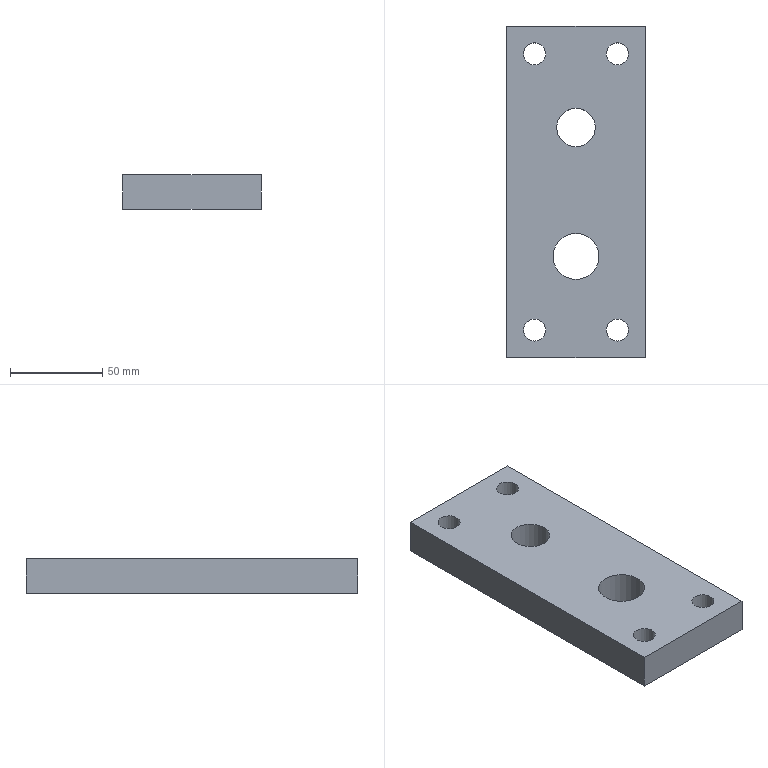Part | NX | features solid 2 | 1 solid | 12 faces | box 75 x 180 x 19 mm | volume 231997 mm3 | plane 6 | cylinder 6 | commonest cylinder face diameters 12 x4 21 x1 25 x1
STEP:
#1=CARTESIAN_POINT('',(-630.,-106.,-55.));
#2=VERTEX_POINT('',#1);
#3=CARTESIAN_POINT('',(-630.,-100.,-55.));
#4=DIRECTION('',(0.,0.,1.));
#5=DIRECTION('',(0.,-1.,0.));
#6=AXIS2_PLACEMENT_3D('',#3,#4,#5);
#7=CIRCLE('',#6,6.);
#8=EDGE_CURVE('',#2,#2,#7,.T.);
#9=ORIENTED_EDGE('',*,*,#8,.F.);
#10=EDGE_LOOP('',(#9));
#11=FACE_BOUND('',#10,.T.);
#12=CARTESIAN_POINT('',(-652.5,-197.5,-55.));
#13=VERTEX_POINT('',#12);
#14=CARTESIAN_POINT('',(-652.5,-210.,-55.));
#15=DIRECTION('',(0.,0.,1.));
#16=DIRECTION('',(0.,1.,0.));
#17=AXIS2_PLACEMENT_3D('',#14,#15,#16);
#18=CIRCLE('',#17,12.5);
#19=EDGE_CURVE('',#13,#13,#18,.T.);
#20=ORIENTED_EDGE('',*,*,#19,.F.);
#21=EDGE_LOOP('',(#20));
#22=FACE_BOUND('',#21,.T.);
#23=CARTESIAN_POINT('',(-652.5,-129.5,-55.));
#24=VERTEX_POINT('',#23);
#25=CARTESIAN_POINT('',(-652.5,-140.,-55.));
#26=DIRECTION('',(0.,0.,1.));
#27=DIRECTION('',(0.,1.,0.));
#28=AXIS2_PLACEMENT_3D('',#25,#26,#27);
#29=CIRCLE('',#28,10.5);
#30=EDGE_CURVE('',#24,#24,#29,.T.);
#31=ORIENTED_EDGE('',*,*,#30,.F.);
#32=EDGE_LOOP('',(#31));
#33=FACE_BOUND('',#32,.T.);
#34=CARTESIAN_POINT('',(-675.,-244.,-55.));
#35=VERTEX_POINT('',#34);
#36=CARTESIAN_POINT('',(-675.,-250.,-55.));
#37=DIRECTION('',(0.,0.,1.));
#38=DIRECTION('',(0.,1.,0.));
#39=AXIS2_PLACEMENT_3D('',#36,#37,#38);
#40=CIRCLE('',#39,6.);
#41=EDGE_CURVE('',#35,#35,#40,.T.);
#42=ORIENTED_EDGE('',*,*,#41,.F.);
#43=EDGE_LOOP('',(#42));
#44=FACE_BOUND('',#43,.T.);
#45=CARTESIAN_POINT('',(-630.,-244.,-55.));
#46=VERTEX_POINT('',#45);
#47=CARTESIAN_POINT('',(-630.,-250.,-55.));
#48=DIRECTION('',(0.,0.,-1.));
#49=DIRECTION('',(0.,1.,0.));
#50=AXIS2_PLACEMENT_3D('',#47,#48,#49);
#51=CIRCLE('',#50,6.);
#52=EDGE_CURVE('',#46,#46,#51,.T.);
#53=ORIENTED_EDGE('',*,*,#52,.T.);
#54=EDGE_LOOP('',(#53));
#55=FACE_BOUND('',#54,.T.);
#56=CARTESIAN_POINT('',(-690.,-85.,-55.));
#57=VERTEX_POINT('',#56);
#58=CARTESIAN_POINT('',(-615.,-85.,-55.));
#59=VERTEX_POINT('',#58);
#60=CARTESIAN_POINT('',(-690.,-85.,-55.));
#61=DIRECTION('',(1.,0.,0.));
#62=VECTOR('',#61,1000.);
#63=LINE('',#60,#62);
#64=EDGE_CURVE('',#57,#59,#63,.T.);
#65=ORIENTED_EDGE('',*,*,#64,.F.);
#66=CARTESIAN_POINT('',(-690.,-265.,-55.));
#67=VERTEX_POINT('',#66);
#68=CARTESIAN_POINT('',(-690.,-15.,-55.));
#69=DIRECTION('',(0.,-1.,0.));
#70=VECTOR('',#69,1000.);
#71=LINE('',#68,#70);
#72=EDGE_CURVE('',#57,#67,#71,.T.);
#73=ORIENTED_EDGE('',*,*,#72,.T.);
#74=CARTESIAN_POINT('',(-615.,-265.,-55.));
#75=VERTEX_POINT('',#74);
#76=CARTESIAN_POINT('',(-690.,-265.,-55.));
#77=DIRECTION('',(1.,0.,0.));
#78=VECTOR('',#77,1000.);
#79=LINE('',#76,#78);
#80=EDGE_CURVE('',#67,#75,#79,.T.);
#81=ORIENTED_EDGE('',*,*,#80,.T.);
#82=CARTESIAN_POINT('',(-615.,-265.,-55.));
#83=DIRECTION('',(0.,1.,0.));
#84=VECTOR('',#83,1000.);
#85=LINE('',#82,#84);
#86=EDGE_CURVE('',#75,#59,#85,.T.);
#87=ORIENTED_EDGE('',*,*,#86,.T.);
#88=EDGE_LOOP('',(#65,#73,#81,#87));
#89=FACE_BOUND('',#88,.T.);
#90=CARTESIAN_POINT('',(-675.,-106.,-55.));
#91=VERTEX_POINT('',#90);
#92=CARTESIAN_POINT('',(-675.,-100.,-55.));
#93=DIRECTION('',(0.,0.,-1.));
#94=DIRECTION('',(0.,-1.,0.));
#95=AXIS2_PLACEMENT_3D('',#92,#93,#94);
#96=CIRCLE('',#95,6.);
#97=EDGE_CURVE('',#91,#91,#96,.T.);
#98=ORIENTED_EDGE('',*,*,#97,.T.);
#99=EDGE_LOOP('',(#98));
#100=FACE_BOUND('',#99,.T.);
#101=CARTESIAN_POINT('',(-690.,-265.,-55.));
#102=DIRECTION('',(0.,0.,1.));
#103=DIRECTION('',(0.,1.,0.));
#104=AXIS2_PLACEMENT_3D('',#101,#102,#103);
#105=PLANE('',#104);
#106=ADVANCED_FACE('',(#11,#22,#33,#44,#55,#89,#100),#105,.T.);
#107=CARTESIAN_POINT('',(-630.,-106.,-74.));
#108=VERTEX_POINT('',#107);
#109=CARTESIAN_POINT('',(-630.,-100.,-74.));
#110=DIRECTION('',(0.,0.,1.));
#111=DIRECTION('',(0.,-1.,0.));
#112=AXIS2_PLACEMENT_3D('',#109,#110,#111);
#113=CIRCLE('',#112,6.);
#114=EDGE_CURVE('',#108,#108,#113,.T.);
#115=ORIENTED_EDGE('',*,*,#114,.T.);
#116=EDGE_LOOP('',(#115));
#117=FACE_BOUND('',#116,.T.);
#118=CARTESIAN_POINT('',(-690.,-85.,-74.));
#119=VERTEX_POINT('',#118);
#120=CARTESIAN_POINT('',(-690.,-265.,-74.));
#121=VERTEX_POINT('',#120);
#122=CARTESIAN_POINT('',(-690.,-15.,-74.));
#123=DIRECTION('',(0.,-1.,0.));
#124=VECTOR('',#123,1000.);
#125=LINE('',#122,#124);
#126=EDGE_CURVE('',#119,#121,#125,.T.);
#127=ORIENTED_EDGE('',*,*,#126,.F.);
#128=CARTESIAN_POINT('',(-615.,-85.,-74.));
#129=VERTEX_POINT('',#128);
#130=CARTESIAN_POINT('',(-690.,-85.,-74.));
#131=DIRECTION('',(1.,0.,0.));
#132=VECTOR('',#131,1000.);
#133=LINE('',#130,#132);
#134=EDGE_CURVE('',#119,#129,#133,.T.);
#135=ORIENTED_EDGE('',*,*,#134,.T.);
#136=CARTESIAN_POINT('',(-615.,-265.,-74.));
#137=VERTEX_POINT('',#136);
#138=CARTESIAN_POINT('',(-615.,-265.,-74.));
#139=DIRECTION('',(0.,1.,0.));
#140=VECTOR('',#139,1000.);
#141=LINE('',#138,#140);
#142=EDGE_CURVE('',#137,#129,#141,.T.);
#143=ORIENTED_EDGE('',*,*,#142,.F.);
#144=CARTESIAN_POINT('',(-690.,-265.,-74.));
#145=DIRECTION('',(1.,0.,0.));
#146=VECTOR('',#145,1000.);
#147=LINE('',#144,#146);
#148=EDGE_CURVE('',#121,#137,#147,.T.);
#149=ORIENTED_EDGE('',*,*,#148,.F.);
#150=EDGE_LOOP('',(#127,#135,#143,#149));
#151=FACE_BOUND('',#150,.T.);
#152=CARTESIAN_POINT('',(-652.5,-197.5,-74.));
#153=VERTEX_POINT('',#152);
#154=CARTESIAN_POINT('',(-652.5,-210.,-74.));
#155=DIRECTION('',(0.,0.,1.));
#156=DIRECTION('',(0.,1.,0.));
#157=AXIS2_PLACEMENT_3D('',#154,#155,#156);
#158=CIRCLE('',#157,12.5);
#159=EDGE_CURVE('',#153,#153,#158,.T.);
#160=ORIENTED_EDGE('',*,*,#159,.T.);
#161=EDGE_LOOP('',(#160));
#162=FACE_BOUND('',#161,.T.);
#163=CARTESIAN_POINT('',(-652.5,-129.5,-74.));
#164=VERTEX_POINT('',#163);
#165=CARTESIAN_POINT('',(-652.5,-140.,-74.));
#166=DIRECTION('',(0.,0.,1.));
#167=DIRECTION('',(0.,1.,0.));
#168=AXIS2_PLACEMENT_3D('',#165,#166,#167);
#169=CIRCLE('',#168,10.5);
#170=EDGE_CURVE('',#164,#164,#169,.T.);
#171=ORIENTED_EDGE('',*,*,#170,.T.);
#172=EDGE_LOOP('',(#171));
#173=FACE_BOUND('',#172,.T.);
#174=CARTESIAN_POINT('',(-675.,-244.,-74.));
#175=VERTEX_POINT('',#174);
#176=CARTESIAN_POINT('',(-675.,-250.,-74.));
#177=DIRECTION('',(0.,0.,1.));
#178=DIRECTION('',(0.,1.,0.));
#179=AXIS2_PLACEMENT_3D('',#176,#177,#178);
#180=CIRCLE('',#179,6.);
#181=EDGE_CURVE('',#175,#175,#180,.T.);
#182=ORIENTED_EDGE('',*,*,#181,.T.);
#183=EDGE_LOOP('',(#182));
#184=FACE_BOUND('',#183,.T.);
#185=CARTESIAN_POINT('',(-630.,-244.,-74.));
#186=VERTEX_POINT('',#185);
#187=CARTESIAN_POINT('',(-630.,-250.,-74.));
#188=DIRECTION('',(0.,0.,-1.));
#189=DIRECTION('',(0.,1.,0.));
#190=AXIS2_PLACEMENT_3D('',#187,#188,#189);
#191=CIRCLE('',#190,6.);
#192=EDGE_CURVE('',#186,#186,#191,.T.);
#193=ORIENTED_EDGE('',*,*,#192,.F.);
#194=EDGE_LOOP('',(#193));
#195=FACE_BOUND('',#194,.T.);
#196=CARTESIAN_POINT('',(-675.,-106.,-74.));
#197=VERTEX_POINT('',#196);
#198=CARTESIAN_POINT('',(-675.,-100.,-74.));
#199=DIRECTION('',(0.,0.,-1.));
#200=DIRECTION('',(0.,-1.,0.));
#201=AXIS2_PLACEMENT_3D('',#198,#199,#200);
#202=CIRCLE('',#201,6.);
#203=EDGE_CURVE('',#197,#197,#202,.T.);
#204=ORIENTED_EDGE('',*,*,#203,.F.);
#205=EDGE_LOOP('',(#204));
#206=FACE_BOUND('',#205,.T.);
#207=CARTESIAN_POINT('',(-690.,-265.,-74.));
#208=DIRECTION('',(0.,0.,1.));
#209=DIRECTION('',(0.,1.,0.));
#210=AXIS2_PLACEMENT_3D('',#207,#208,#209);
#211=PLANE('',#210);
#212=ADVANCED_FACE('',(#117,#151,#162,#173,#184,#195,#206),#211,.F.);
#213=CARTESIAN_POINT('',(-690.,-85.,-55.));
#214=DIRECTION('',(0.,0.,-1.));
#215=VECTOR('',#214,1000.);
#216=LINE('',#213,#215);
#217=EDGE_CURVE('',#57,#119,#216,.T.);
#218=ORIENTED_EDGE('',*,*,#217,.F.);
#219=ORIENTED_EDGE('',*,*,#64,.T.);
#220=CARTESIAN_POINT('',(-615.,-85.,-55.));
#221=DIRECTION('',(0.,0.,1.));
#222=VECTOR('',#221,1000.);
#223=LINE('',#220,#222);
#224=EDGE_CURVE('',#129,#59,#223,.T.);
#225=ORIENTED_EDGE('',*,*,#224,.F.);
#226=ORIENTED_EDGE('',*,*,#134,.F.);
#227=EDGE_LOOP('',(#218,#219,#225,#226));
#228=FACE_BOUND('',#227,.T.);
#229=CARTESIAN_POINT('',(-652.5,-85.,-64.5));
#230=DIRECTION('',(0.,-1.,0.));
#231=DIRECTION('',(0.,0.,1.));
#232=AXIS2_PLACEMENT_3D('',#229,#230,#231);
#233=PLANE('',#232);
#234=ADVANCED_FACE('',(#228),#233,.F.);
#235=ORIENTED_EDGE('',*,*,#72,.F.);
#236=ORIENTED_EDGE('',*,*,#217,.T.);
#237=ORIENTED_EDGE('',*,*,#126,.T.);
#238=CARTESIAN_POINT('',(-690.,-265.,-55.));
#239=DIRECTION('',(0.,0.,-1.));
#240=VECTOR('',#239,1000.);
#241=LINE('',#238,#240);
#242=EDGE_CURVE('',#67,#121,#241,.T.);
#243=ORIENTED_EDGE('',*,*,#242,.F.);
#244=EDGE_LOOP('',(#235,#236,#237,#243));
#245=FACE_BOUND('',#244,.T.);
#246=CARTESIAN_POINT('',(-690.,-15.,-55.));
#247=DIRECTION('',(1.,0.,0.));
#248=DIRECTION('',(0.,1.,0.));
#249=AXIS2_PLACEMENT_3D('',#246,#247,#248);
#250=PLANE('',#249);
#251=ADVANCED_FACE('',(#245),#250,.F.);
#252=ORIENTED_EDGE('',*,*,#142,.T.);
#253=ORIENTED_EDGE('',*,*,#224,.T.);
#254=ORIENTED_EDGE('',*,*,#86,.F.);
#255=CARTESIAN_POINT('',(-615.,-265.,-55.));
#256=DIRECTION('',(0.,0.,-1.));
#257=VECTOR('',#256,1000.);
#258=LINE('',#255,#257);
#259=EDGE_CURVE('',#75,#137,#258,.T.);
#260=ORIENTED_EDGE('',*,*,#259,.T.);
#261=EDGE_LOOP('',(#252,#253,#254,#260));
#262=FACE_BOUND('',#261,.T.);
#263=CARTESIAN_POINT('',(-615.,-265.,-55.));
#264=DIRECTION('',(-1.,0.,0.));
#265=DIRECTION('',(0.,-1.,0.));
#266=AXIS2_PLACEMENT_3D('',#263,#264,#265);
#267=PLANE('',#266);
#268=ADVANCED_FACE('',(#262),#267,.F.);
#269=ORIENTED_EDGE('',*,*,#148,.T.);
#270=ORIENTED_EDGE('',*,*,#259,.F.);
#271=ORIENTED_EDGE('',*,*,#80,.F.);
#272=ORIENTED_EDGE('',*,*,#242,.T.);
#273=EDGE_LOOP('',(#269,#270,#271,#272));
#274=FACE_BOUND('',#273,.T.);
#275=CARTESIAN_POINT('',(-690.,-265.,-55.));
#276=DIRECTION('',(0.,1.,0.));
#277=DIRECTION('',(0.,0.,-1.));
#278=AXIS2_PLACEMENT_3D('',#275,#276,#277);
#279=PLANE('',#278);
#280=ADVANCED_FACE('',(#274),#279,.F.);
#281=ORIENTED_EDGE('',*,*,#41,.T.);
#282=EDGE_LOOP('',(#281));
#283=FACE_BOUND('',#282,.T.);
#284=ORIENTED_EDGE('',*,*,#181,.F.);
#285=EDGE_LOOP('',(#284));
#286=FACE_BOUND('',#285,.T.);
#287=CARTESIAN_POINT('',(-675.,-250.,-55.));
#288=DIRECTION('',(0.,0.,-1.));
#289=DIRECTION('',(0.,-1.,0.));
#290=AXIS2_PLACEMENT_3D('',#287,#288,#289);
#291=CYLINDRICAL_SURFACE('',#290,6.);
#292=ADVANCED_FACE('',(#283,#286),#291,.F.);
#293=ORIENTED_EDGE('',*,*,#30,.T.);
#294=EDGE_LOOP('',(#293));
#295=FACE_BOUND('',#294,.T.);
#296=ORIENTED_EDGE('',*,*,#170,.F.);
#297=EDGE_LOOP('',(#296));
#298=FACE_BOUND('',#297,.T.);
#299=CARTESIAN_POINT('',(-652.5,-140.,-55.));
#300=DIRECTION('',(0.,0.,-1.));
#301=DIRECTION('',(0.,-1.,0.));
#302=AXIS2_PLACEMENT_3D('',#299,#300,#301);
#303=CYLINDRICAL_SURFACE('',#302,10.5);
#304=ADVANCED_FACE('',(#295,#298),#303,.F.);
#305=ORIENTED_EDGE('',*,*,#19,.T.);
#306=EDGE_LOOP('',(#305));
#307=FACE_BOUND('',#306,.T.);
#308=ORIENTED_EDGE('',*,*,#159,.F.);
#309=EDGE_LOOP('',(#308));
#310=FACE_BOUND('',#309,.T.);
#311=CARTESIAN_POINT('',(-652.5,-210.,-55.));
#312=DIRECTION('',(0.,0.,-1.));
#313=DIRECTION('',(0.,-1.,0.));
#314=AXIS2_PLACEMENT_3D('',#311,#312,#313);
#315=CYLINDRICAL_SURFACE('',#314,12.5);
#316=ADVANCED_FACE('',(#307,#310),#315,.F.);
#317=ORIENTED_EDGE('',*,*,#52,.F.);
#318=EDGE_LOOP('',(#317));
#319=FACE_BOUND('',#318,.T.);
#320=ORIENTED_EDGE('',*,*,#192,.T.);
#321=EDGE_LOOP('',(#320));
#322=FACE_BOUND('',#321,.T.);
#323=CARTESIAN_POINT('',(-630.,-250.,-55.));
#324=DIRECTION('',(0.,0.,-1.));
#325=DIRECTION('',(0.,-1.,0.));
#326=AXIS2_PLACEMENT_3D('',#323,#324,#325);
#327=CYLINDRICAL_SURFACE('',#326,6.);
#328=ADVANCED_FACE('',(#319,#322),#327,.F.);
#329=ORIENTED_EDGE('',*,*,#97,.F.);
#330=EDGE_LOOP('',(#329));
#331=FACE_BOUND('',#330,.T.);
#332=ORIENTED_EDGE('',*,*,#203,.T.);
#333=EDGE_LOOP('',(#332));
#334=FACE_BOUND('',#333,.T.);
#335=CARTESIAN_POINT('',(-675.,-100.,-55.));
#336=DIRECTION('',(0.,0.,-1.));
#337=DIRECTION('',(0.,1.,0.));
#338=AXIS2_PLACEMENT_3D('',#335,#336,#337);
#339=CYLINDRICAL_SURFACE('',#338,6.);
#340=ADVANCED_FACE('',(#331,#334),#339,.F.);
#341=ORIENTED_EDGE('',*,*,#8,.T.);
#342=EDGE_LOOP('',(#341));
#343=FACE_BOUND('',#342,.T.);
#344=ORIENTED_EDGE('',*,*,#114,.F.);
#345=EDGE_LOOP('',(#344));
#346=FACE_BOUND('',#345,.T.);
#347=CARTESIAN_POINT('',(-630.,-100.,-55.));
#348=DIRECTION('',(0.,0.,-1.));
#349=DIRECTION('',(0.,1.,0.));
#350=AXIS2_PLACEMENT_3D('',#347,#348,#349);
#351=CYLINDRICAL_SURFACE('',#350,6.);
#352=ADVANCED_FACE('',(#343,#346),#351,.F.);
#353=CLOSED_SHELL('',(#106,#212,#234,#251,#268,#280,#292,#304,#316,#328,#340,#352));
#354=MANIFOLD_SOLID_BREP('',#353);
#355=(LENGTH_UNIT()NAMED_UNIT(*)SI_UNIT(.MILLI.,.METRE.));
#356=UNCERTAINTY_MEASURE_WITH_UNIT(LENGTH_MEASURE(0.00001),#355,'','');
#357=(NAMED_UNIT(*)PLANE_ANGLE_UNIT()SI_UNIT($,.RADIAN.));
#358=(NAMED_UNIT(*)SI_UNIT($,.STERADIAN.)SOLID_ANGLE_UNIT());
#359=(GEOMETRIC_REPRESENTATION_CONTEXT(3)GLOBAL_UNCERTAINTY_ASSIGNED_CONTEXT((#356))GLOBAL_UNIT_ASSIGNED_CONTEXT((#355,#357,#358))REPRESENTATION_CONTEXT('',''));
#360=ADVANCED_BREP_SHAPE_REPRESENTATION('',(#354),#359);